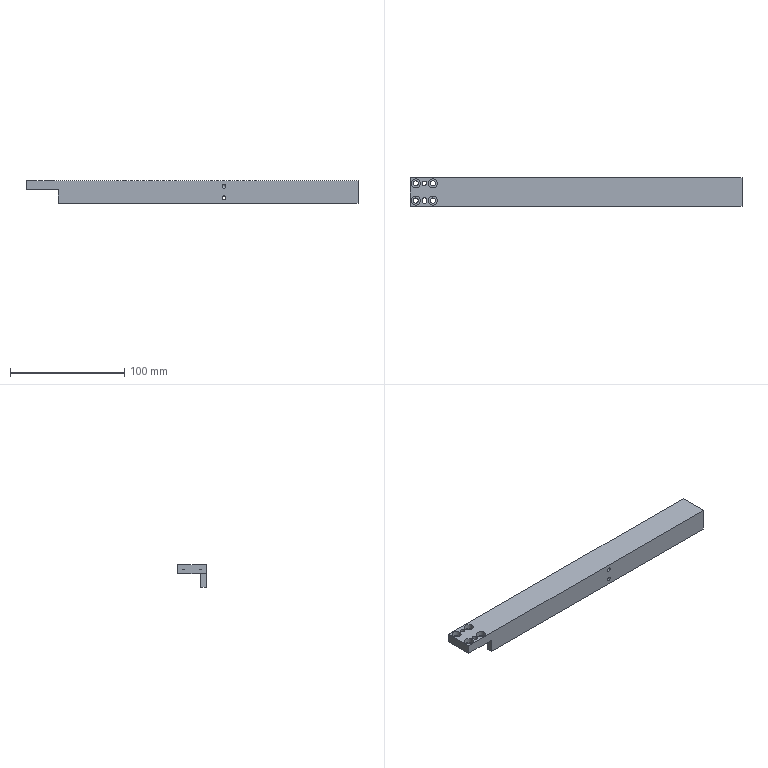Part | NX | 1 solid | 31 faces | box 290 x 25 x 20 mm | volume 71804 mm3 | plane 17 | cylinder 13 | cone 1 | commonest cylinder face diameters 4.5 x4 8 x4 4 x3 3.3 x2
STEP:
#1=CARTESIAN_POINT('',(-117.,-7.5,-20.));
#2=VERTEX_POINT('',#1);
#3=CARTESIAN_POINT('',(136.758,-7.5,-20.));
#4=VERTEX_POINT('',#3);
#5=CARTESIAN_POINT('',(-145.,-7.5,-20.));
#6=DIRECTION('',(1.,0.,0.));
#7=VECTOR('',#6,1000.);
#8=LINE('',#5,#7);
#9=EDGE_CURVE('',#2,#4,#8,.T.);
#10=ORIENTED_EDGE('',*,*,#9,.T.);
#11=CARTESIAN_POINT('',(145.,-10.5,-20.));
#12=VERTEX_POINT('',#11);
#13=CARTESIAN_POINT('',(136.758,-7.5,-20.));
#14=DIRECTION('',(0.9397,-0.342,0.));
#15=VECTOR('',#14,1000.);
#16=LINE('',#13,#15);
#17=EDGE_CURVE('',#4,#12,#16,.T.);
#18=ORIENTED_EDGE('',*,*,#17,.T.);
#19=CARTESIAN_POINT('',(145.,-12.5,-20.));
#20=VERTEX_POINT('',#19);
#21=CARTESIAN_POINT('',(145.,12.5,-20.));
#22=DIRECTION('',(0.,-1.,0.));
#23=VECTOR('',#22,1000.);
#24=LINE('',#21,#23);
#25=EDGE_CURVE('',#12,#20,#24,.T.);
#26=ORIENTED_EDGE('',*,*,#25,.T.);
#27=CARTESIAN_POINT('',(-117.,-12.5,-20.));
#28=VERTEX_POINT('',#27);
#29=CARTESIAN_POINT('',(145.,-12.5,-20.));
#30=DIRECTION('',(-1.,0.,0.));
#31=VECTOR('',#30,1000.);
#32=LINE('',#29,#31);
#33=EDGE_CURVE('',#20,#28,#32,.T.);
#34=ORIENTED_EDGE('',*,*,#33,.T.);
#35=CARTESIAN_POINT('',(-117.,-12.5,-20.));
#36=DIRECTION('',(0.,1.,0.));
#37=VECTOR('',#36,1000.);
#38=LINE('',#35,#37);
#39=EDGE_CURVE('',#28,#2,#38,.T.);
#40=ORIENTED_EDGE('',*,*,#39,.T.);
#41=EDGE_LOOP('',(#10,#18,#26,#34,#40));
#42=FACE_BOUND('',#41,.T.);
#43=CARTESIAN_POINT('',(145.,12.5,-20.));
#44=DIRECTION('',(0.,0.,1.));
#45=DIRECTION('',(-1.,0.,0.));
#46=AXIS2_PLACEMENT_3D('',#43,#44,#45);
#47=PLANE('',#46);
#48=ADVANCED_FACE('',(#42),#47,.F.);
#49=CARTESIAN_POINT('',(-145.,12.5,-8.));
#50=VERTEX_POINT('',#49);
#51=CARTESIAN_POINT('',(-145.,-12.5,-8.));
#52=VERTEX_POINT('',#51);
#53=CARTESIAN_POINT('',(-145.,-7.5,-8.));
#54=DIRECTION('',(0.,-1.,0.));
#55=VECTOR('',#54,1000.);
#56=LINE('',#53,#55);
#57=EDGE_CURVE('',#50,#52,#56,.T.);
#58=ORIENTED_EDGE('',*,*,#57,.T.);
#59=CARTESIAN_POINT('',(-145.,-12.5,0.));
#60=VERTEX_POINT('',#59);
#61=CARTESIAN_POINT('',(-145.,-12.5,-20.));
#62=DIRECTION('',(0.,0.,1.));
#63=VECTOR('',#62,1000.);
#64=LINE('',#61,#63);
#65=EDGE_CURVE('',#52,#60,#64,.T.);
#66=ORIENTED_EDGE('',*,*,#65,.T.);
#67=CARTESIAN_POINT('',(-145.,12.5,0.));
#68=VERTEX_POINT('',#67);
#69=CARTESIAN_POINT('',(-145.,12.5,0.));
#70=DIRECTION('',(0.,-1.,0.));
#71=VECTOR('',#70,1000.);
#72=LINE('',#69,#71);
#73=EDGE_CURVE('',#68,#60,#72,.T.);
#74=ORIENTED_EDGE('',*,*,#73,.F.);
#75=CARTESIAN_POINT('',(-145.,12.5,-20.));
#76=DIRECTION('',(0.,0.,1.));
#77=VECTOR('',#76,1000.);
#78=LINE('',#75,#77);
#79=EDGE_CURVE('',#50,#68,#78,.T.);
#80=ORIENTED_EDGE('',*,*,#79,.F.);
#81=EDGE_LOOP('',(#58,#66,#74,#80));
#82=FACE_BOUND('',#81,.T.);
#83=CARTESIAN_POINT('',(-145.,12.5,-20.));
#84=DIRECTION('',(1.,0.,0.));
#85=DIRECTION('',(0.,0.,1.));
#86=AXIS2_PLACEMENT_3D('',#83,#84,#85);
#87=PLANE('',#86);
#88=ADVANCED_FACE('',(#82),#87,.F.);
#89=CARTESIAN_POINT('',(-134.5,-7.,0.));
#90=VERTEX_POINT('',#89);
#91=CARTESIAN_POINT('',(-134.5,-8.,0.));
#92=VERTEX_POINT('',#91);
#93=CARTESIAN_POINT('',(-134.5,-7.,0.));
#94=DIRECTION('',(0.,-1.,0.));
#95=VECTOR('',#94,1000.);
#96=LINE('',#93,#95);
#97=EDGE_CURVE('',#90,#92,#96,.T.);
#98=ORIENTED_EDGE('',*,*,#97,.F.);
#99=CARTESIAN_POINT('',(-130.5,-7.,0.));
#100=VERTEX_POINT('',#99);
#101=CARTESIAN_POINT('',(-132.5,-7.,0.));
#102=DIRECTION('',(0.,0.,1.));
#103=DIRECTION('',(1.,0.,0.));
#104=AXIS2_PLACEMENT_3D('',#101,#102,#103);
#105=CIRCLE('',#104,2.);
#106=EDGE_CURVE('',#100,#90,#105,.T.);
#107=ORIENTED_EDGE('',*,*,#106,.F.);
#108=CARTESIAN_POINT('',(-130.5,-8.,0.));
#109=VERTEX_POINT('',#108);
#110=CARTESIAN_POINT('',(-130.5,-7.,0.));
#111=DIRECTION('',(0.,1.,0.));
#112=VECTOR('',#111,1000.);
#113=LINE('',#110,#112);
#114=EDGE_CURVE('',#109,#100,#113,.T.);
#115=ORIENTED_EDGE('',*,*,#114,.F.);
#116=CARTESIAN_POINT('',(-132.5,-8.,0.));
#117=DIRECTION('',(0.,0.,1.));
#118=DIRECTION('',(1.,0.,0.));
#119=AXIS2_PLACEMENT_3D('',#116,#117,#118);
#120=CIRCLE('',#119,2.);
#121=EDGE_CURVE('',#92,#109,#120,.T.);
#122=ORIENTED_EDGE('',*,*,#121,.F.);
#123=EDGE_LOOP('',(#98,#107,#115,#122));
#124=FACE_BOUND('',#123,.T.);
#125=CARTESIAN_POINT('',(-130.5,7.5,0.));
#126=VERTEX_POINT('',#125);
#127=CARTESIAN_POINT('',(-132.5,7.5,0.));
#128=DIRECTION('',(0.,0.,1.));
#129=DIRECTION('',(1.,0.,0.));
#130=AXIS2_PLACEMENT_3D('',#127,#128,#129);
#131=CIRCLE('',#130,2.);
#132=EDGE_CURVE('',#126,#126,#131,.T.);
#133=ORIENTED_EDGE('',*,*,#132,.F.);
#134=EDGE_LOOP('',(#133));
#135=FACE_BOUND('',#134,.T.);
#136=CARTESIAN_POINT('',(-136.,7.5,0.));
#137=VERTEX_POINT('',#136);
#138=CARTESIAN_POINT('',(-140.,7.5,0.));
#139=DIRECTION('',(0.,0.,1.));
#140=DIRECTION('',(1.,0.,0.));
#141=AXIS2_PLACEMENT_3D('',#138,#139,#140);
#142=CIRCLE('',#141,4.);
#143=EDGE_CURVE('',#137,#137,#142,.T.);
#144=ORIENTED_EDGE('',*,*,#143,.F.);
#145=EDGE_LOOP('',(#144));
#146=FACE_BOUND('',#145,.T.);
#147=CARTESIAN_POINT('',(-136.,-7.5,0.));
#148=VERTEX_POINT('',#147);
#149=CARTESIAN_POINT('',(-140.,-7.5,0.));
#150=DIRECTION('',(0.,0.,1.));
#151=DIRECTION('',(1.,0.,0.));
#152=AXIS2_PLACEMENT_3D('',#149,#150,#151);
#153=CIRCLE('',#152,4.);
#154=EDGE_CURVE('',#148,#148,#153,.T.);
#155=ORIENTED_EDGE('',*,*,#154,.F.);
#156=EDGE_LOOP('',(#155));
#157=FACE_BOUND('',#156,.T.);
#158=CARTESIAN_POINT('',(-121.,-7.5,0.));
#159=VERTEX_POINT('',#158);
#160=CARTESIAN_POINT('',(-125.,-7.5,0.));
#161=DIRECTION('',(0.,0.,1.));
#162=DIRECTION('',(1.,0.,0.));
#163=AXIS2_PLACEMENT_3D('',#160,#161,#162);
#164=CIRCLE('',#163,4.);
#165=EDGE_CURVE('',#159,#159,#164,.T.);
#166=ORIENTED_EDGE('',*,*,#165,.F.);
#167=EDGE_LOOP('',(#166));
#168=FACE_BOUND('',#167,.T.);
#169=CARTESIAN_POINT('',(-121.,7.5,0.));
#170=VERTEX_POINT('',#169);
#171=CARTESIAN_POINT('',(-125.,7.5,0.));
#172=DIRECTION('',(0.,0.,1.));
#173=DIRECTION('',(1.,0.,0.));
#174=AXIS2_PLACEMENT_3D('',#171,#172,#173);
#175=CIRCLE('',#174,4.);
#176=EDGE_CURVE('',#170,#170,#175,.T.);
#177=ORIENTED_EDGE('',*,*,#176,.F.);
#178=EDGE_LOOP('',(#177));
#179=FACE_BOUND('',#178,.T.);
#180=CARTESIAN_POINT('',(145.,-12.5,0.));
#181=VERTEX_POINT('',#180);
#182=CARTESIAN_POINT('',(145.,-12.5,0.));
#183=DIRECTION('',(1.,0.,0.));
#184=VECTOR('',#183,1000.);
#185=LINE('',#182,#184);
#186=EDGE_CURVE('',#60,#181,#185,.T.);
#187=ORIENTED_EDGE('',*,*,#186,.T.);
#188=CARTESIAN_POINT('',(145.,12.5,0.));
#189=VERTEX_POINT('',#188);
#190=CARTESIAN_POINT('',(145.,12.5,0.));
#191=DIRECTION('',(0.,-1.,0.));
#192=VECTOR('',#191,1000.);
#193=LINE('',#190,#192);
#194=EDGE_CURVE('',#189,#181,#193,.T.);
#195=ORIENTED_EDGE('',*,*,#194,.F.);
#196=CARTESIAN_POINT('',(145.,12.5,0.));
#197=DIRECTION('',(1.,0.,0.));
#198=VECTOR('',#197,1000.);
#199=LINE('',#196,#198);
#200=EDGE_CURVE('',#68,#189,#199,.T.);
#201=ORIENTED_EDGE('',*,*,#200,.F.);
#202=ORIENTED_EDGE('',*,*,#73,.T.);
#203=EDGE_LOOP('',(#187,#195,#201,#202));
#204=FACE_BOUND('',#203,.T.);
#205=CARTESIAN_POINT('',(145.,12.5,0.));
#206=DIRECTION('',(0.,0.,-1.));
#207=DIRECTION('',(1.,0.,0.));
#208=AXIS2_PLACEMENT_3D('',#205,#206,#207);
#209=PLANE('',#208);
#210=ADVANCED_FACE('',(#124,#135,#146,#157,#168,#179,#204),#209,.F.);
#211=ORIENTED_EDGE('',*,*,#25,.F.);
#212=CARTESIAN_POINT('',(145.,-10.5,-5.));
#213=VERTEX_POINT('',#212);
#214=CARTESIAN_POINT('',(145.,-10.5,-20.));
#215=DIRECTION('',(0.,0.,1.));
#216=VECTOR('',#215,1000.);
#217=LINE('',#214,#216);
#218=EDGE_CURVE('',#12,#213,#217,.T.);
#219=ORIENTED_EDGE('',*,*,#218,.T.);
#220=CARTESIAN_POINT('',(145.,12.5,-5.));
#221=VERTEX_POINT('',#220);
#222=CARTESIAN_POINT('',(145.,12.5,-5.));
#223=DIRECTION('',(0.,1.,0.));
#224=VECTOR('',#223,1000.);
#225=LINE('',#222,#224);
#226=EDGE_CURVE('',#213,#221,#225,.T.);
#227=ORIENTED_EDGE('',*,*,#226,.T.);
#228=CARTESIAN_POINT('',(145.,12.5,-20.));
#229=DIRECTION('',(0.,0.,-1.));
#230=VECTOR('',#229,1000.);
#231=LINE('',#228,#230);
#232=EDGE_CURVE('',#189,#221,#231,.T.);
#233=ORIENTED_EDGE('',*,*,#232,.F.);
#234=ORIENTED_EDGE('',*,*,#194,.T.);
#235=CARTESIAN_POINT('',(145.,-12.5,-20.));
#236=DIRECTION('',(0.,0.,-1.));
#237=VECTOR('',#236,1000.);
#238=LINE('',#235,#237);
#239=EDGE_CURVE('',#181,#20,#238,.T.);
#240=ORIENTED_EDGE('',*,*,#239,.T.);
#241=EDGE_LOOP('',(#211,#219,#227,#233,#234,#240));
#242=FACE_BOUND('',#241,.T.);
#243=CARTESIAN_POINT('',(145.,12.5,-20.));
#244=DIRECTION('',(-1.,0.,0.));
#245=DIRECTION('',(0.,0.,-1.));
#246=AXIS2_PLACEMENT_3D('',#243,#244,#245);
#247=PLANE('',#246);
#248=ADVANCED_FACE('',(#242),#247,.F.);
#249=ORIENTED_EDGE('',*,*,#232,.T.);
#250=CARTESIAN_POINT('',(136.758,12.5,-8.));
#251=VERTEX_POINT('',#250);
#252=CARTESIAN_POINT('',(-115.897,12.5,-99.959));
#253=DIRECTION('',(-0.9397,0.,-0.342));
#254=VECTOR('',#253,1000.);
#255=LINE('',#252,#254);
#256=EDGE_CURVE('',#221,#251,#255,.T.);
#257=ORIENTED_EDGE('',*,*,#256,.T.);
#258=CARTESIAN_POINT('',(-145.,12.5,-8.));
#259=DIRECTION('',(1.,0.,0.));
#260=VECTOR('',#259,1000.);
#261=LINE('',#258,#260);
#262=EDGE_CURVE('',#50,#251,#261,.T.);
#263=ORIENTED_EDGE('',*,*,#262,.F.);
#264=ORIENTED_EDGE('',*,*,#79,.T.);
#265=ORIENTED_EDGE('',*,*,#200,.T.);
#266=EDGE_LOOP('',(#249,#257,#263,#264,#265));
#267=FACE_BOUND('',#266,.T.);
#268=CARTESIAN_POINT('',(-145.,12.5,-20.));
#269=DIRECTION('',(0.,1.,0.));
#270=DIRECTION('',(1.,0.,0.));
#271=AXIS2_PLACEMENT_3D('',#268,#269,#270);
#272=PLANE('',#271);
#273=ADVANCED_FACE('',(#267),#272,.T.);
#274=CARTESIAN_POINT('',(29.65,-12.5,-5.));
#275=VERTEX_POINT('',#274);
#276=CARTESIAN_POINT('',(28.,-12.5,-5.));
#277=DIRECTION('',(0.,-1.,0.));
#278=DIRECTION('',(1.,0.,0.));
#279=AXIS2_PLACEMENT_3D('',#276,#277,#278);
#280=CIRCLE('',#279,1.65);
#281=EDGE_CURVE('',#275,#275,#280,.T.);
#282=ORIENTED_EDGE('',*,*,#281,.F.);
#283=EDGE_LOOP('',(#282));
#284=FACE_BOUND('',#283,.T.);
#285=CARTESIAN_POINT('',(29.65,-12.5,-15.));
#286=VERTEX_POINT('',#285);
#287=CARTESIAN_POINT('',(28.,-12.5,-15.));
#288=DIRECTION('',(0.,-1.,0.));
#289=DIRECTION('',(1.,0.,0.));
#290=AXIS2_PLACEMENT_3D('',#287,#288,#289);
#291=CIRCLE('',#290,1.65);
#292=EDGE_CURVE('',#286,#286,#291,.T.);
#293=ORIENTED_EDGE('',*,*,#292,.F.);
#294=EDGE_LOOP('',(#293));
#295=FACE_BOUND('',#294,.T.);
#296=CARTESIAN_POINT('',(-117.,-12.5,-8.));
#297=VERTEX_POINT('',#296);
#298=CARTESIAN_POINT('',(-145.,-12.5,-8.));
#299=DIRECTION('',(1.,0.,0.));
#300=VECTOR('',#299,1000.);
#301=LINE('',#298,#300);
#302=EDGE_CURVE('',#52,#297,#301,.T.);
#303=ORIENTED_EDGE('',*,*,#302,.T.);
#304=CARTESIAN_POINT('',(-117.,-12.5,-20.));
#305=DIRECTION('',(0.,0.,-1.));
#306=VECTOR('',#305,1000.);
#307=LINE('',#304,#306);
#308=EDGE_CURVE('',#297,#28,#307,.T.);
#309=ORIENTED_EDGE('',*,*,#308,.T.);
#310=ORIENTED_EDGE('',*,*,#33,.F.);
#311=ORIENTED_EDGE('',*,*,#239,.F.);
#312=ORIENTED_EDGE('',*,*,#186,.F.);
#313=ORIENTED_EDGE('',*,*,#65,.F.);
#314=EDGE_LOOP('',(#303,#309,#310,#311,#312,#313));
#315=FACE_BOUND('',#314,.T.);
#316=CARTESIAN_POINT('',(-145.,-12.5,-20.));
#317=DIRECTION('',(0.,1.,0.));
#318=DIRECTION('',(1.,0.,0.));
#319=AXIS2_PLACEMENT_3D('',#316,#317,#318);
#320=PLANE('',#319);
#321=ADVANCED_FACE('',(#284,#295,#315),#320,.F.);
#322=CARTESIAN_POINT('',(28.,-7.5,-13.35));
#323=VERTEX_POINT('',#322);
#324=CARTESIAN_POINT('',(28.,-7.5,-15.));
#325=DIRECTION('',(0.,-1.,0.));
#326=DIRECTION('',(0.,0.,1.));
#327=AXIS2_PLACEMENT_3D('',#324,#325,#326);
#328=CIRCLE('',#327,1.65);
#329=EDGE_CURVE('',#323,#323,#328,.T.);
#330=ORIENTED_EDGE('',*,*,#329,.T.);
#331=EDGE_LOOP('',(#330));
#332=FACE_BOUND('',#331,.T.);
#333=CARTESIAN_POINT('',(-117.,-7.5,-8.));
#334=VERTEX_POINT('',#333);
#335=CARTESIAN_POINT('',(136.758,-7.5,-8.));
#336=VERTEX_POINT('',#335);
#337=CARTESIAN_POINT('',(-145.,-7.5,-8.));
#338=DIRECTION('',(1.,0.,0.));
#339=VECTOR('',#338,1000.);
#340=LINE('',#337,#339);
#341=EDGE_CURVE('',#334,#336,#340,.T.);
#342=ORIENTED_EDGE('',*,*,#341,.T.);
#343=CARTESIAN_POINT('',(136.758,-7.5,-20.));
#344=DIRECTION('',(0.,0.,-1.));
#345=VECTOR('',#344,1000.);
#346=LINE('',#343,#345);
#347=EDGE_CURVE('',#336,#4,#346,.T.);
#348=ORIENTED_EDGE('',*,*,#347,.T.);
#349=ORIENTED_EDGE('',*,*,#9,.F.);
#350=CARTESIAN_POINT('',(-117.,-7.5,-20.));
#351=DIRECTION('',(0.,0.,1.));
#352=VECTOR('',#351,1000.);
#353=LINE('',#350,#352);
#354=EDGE_CURVE('',#2,#334,#353,.T.);
#355=ORIENTED_EDGE('',*,*,#354,.T.);
#356=EDGE_LOOP('',(#342,#348,#349,#355));
#357=FACE_BOUND('',#356,.T.);
#358=CARTESIAN_POINT('',(-145.,-7.5,-20.));
#359=DIRECTION('',(0.,-1.,0.));
#360=DIRECTION('',(0.,0.,-1.));
#361=AXIS2_PLACEMENT_3D('',#358,#359,#360);
#362=PLANE('',#361);
#363=ADVANCED_FACE('',(#332,#357),#362,.F.);
#364=CARTESIAN_POINT('',(-130.5,-8.,-8.));
#365=VERTEX_POINT('',#364);
#366=CARTESIAN_POINT('',(-130.5,-7.,-8.));
#367=VERTEX_POINT('',#366);
#368=CARTESIAN_POINT('',(-130.5,-7.5,-8.));
#369=DIRECTION('',(0.,1.,0.));
#370=VECTOR('',#369,1000.);
#371=LINE('',#368,#370);
#372=EDGE_CURVE('',#365,#367,#371,.T.);
#373=ORIENTED_EDGE('',*,*,#372,.T.);
#374=CARTESIAN_POINT('',(-134.5,-7.,-8.));
#375=VERTEX_POINT('',#374);
#376=CARTESIAN_POINT('',(-132.5,-7.,-8.));
#377=DIRECTION('',(0.,0.,1.));
#378=DIRECTION('',(0.,1.,0.));
#379=AXIS2_PLACEMENT_3D('',#376,#377,#378);
#380=CIRCLE('',#379,2.);
#381=EDGE_CURVE('',#367,#375,#380,.T.);
#382=ORIENTED_EDGE('',*,*,#381,.T.);
#383=CARTESIAN_POINT('',(-134.5,-8.,-8.));
#384=VERTEX_POINT('',#383);
#385=CARTESIAN_POINT('',(-134.5,-7.5,-8.));
#386=DIRECTION('',(0.,-1.,0.));
#387=VECTOR('',#386,1000.);
#388=LINE('',#385,#387);
#389=EDGE_CURVE('',#375,#384,#388,.T.);
#390=ORIENTED_EDGE('',*,*,#389,.T.);
#391=CARTESIAN_POINT('',(-132.5,-8.,-8.));
#392=DIRECTION('',(0.,0.,1.));
#393=DIRECTION('',(0.,1.,0.));
#394=AXIS2_PLACEMENT_3D('',#391,#392,#393);
#395=CIRCLE('',#394,2.);
#396=EDGE_CURVE('',#384,#365,#395,.T.);
#397=ORIENTED_EDGE('',*,*,#396,.T.);
#398=EDGE_LOOP('',(#373,#382,#390,#397));
#399=FACE_BOUND('',#398,.T.);
#400=CARTESIAN_POINT('',(-132.5,9.5,-8.));
#401=VERTEX_POINT('',#400);
#402=CARTESIAN_POINT('',(-132.5,7.5,-8.));
#403=DIRECTION('',(0.,0.,1.));
#404=DIRECTION('',(0.,1.,0.));
#405=AXIS2_PLACEMENT_3D('',#402,#403,#404);
#406=CIRCLE('',#405,2.);
#407=EDGE_CURVE('',#401,#401,#406,.T.);
#408=ORIENTED_EDGE('',*,*,#407,.T.);
#409=EDGE_LOOP('',(#408));
#410=FACE_BOUND('',#409,.T.);
#411=CARTESIAN_POINT('',(-140.,9.75,-8.));
#412=VERTEX_POINT('',#411);
#413=CARTESIAN_POINT('',(-140.,7.5,-8.));
#414=DIRECTION('',(0.,0.,1.));
#415=DIRECTION('',(0.,1.,0.));
#416=AXIS2_PLACEMENT_3D('',#413,#414,#415);
#417=CIRCLE('',#416,2.25);
#418=EDGE_CURVE('',#412,#412,#417,.T.);
#419=ORIENTED_EDGE('',*,*,#418,.T.);
#420=EDGE_LOOP('',(#419));
#421=FACE_BOUND('',#420,.T.);
#422=CARTESIAN_POINT('',(-140.,-5.25,-8.));
#423=VERTEX_POINT('',#422);
#424=CARTESIAN_POINT('',(-140.,-7.5,-8.));
#425=DIRECTION('',(0.,0.,1.));
#426=DIRECTION('',(0.,1.,0.));
#427=AXIS2_PLACEMENT_3D('',#424,#425,#426);
#428=CIRCLE('',#427,2.25);
#429=EDGE_CURVE('',#423,#423,#428,.T.);
#430=ORIENTED_EDGE('',*,*,#429,.T.);
#431=EDGE_LOOP('',(#430));
#432=FACE_BOUND('',#431,.T.);
#433=CARTESIAN_POINT('',(-125.,-5.25,-8.));
#434=VERTEX_POINT('',#433);
#435=CARTESIAN_POINT('',(-125.,-7.5,-8.));
#436=DIRECTION('',(0.,0.,1.));
#437=DIRECTION('',(0.,1.,0.));
#438=AXIS2_PLACEMENT_3D('',#435,#436,#437);
#439=CIRCLE('',#438,2.25);
#440=EDGE_CURVE('',#434,#434,#439,.T.);
#441=ORIENTED_EDGE('',*,*,#440,.T.);
#442=EDGE_LOOP('',(#441));
#443=FACE_BOUND('',#442,.T.);
#444=CARTESIAN_POINT('',(-125.,9.75,-8.));
#445=VERTEX_POINT('',#444);
#446=CARTESIAN_POINT('',(-125.,7.5,-8.));
#447=DIRECTION('',(0.,0.,1.));
#448=DIRECTION('',(0.,1.,0.));
#449=AXIS2_PLACEMENT_3D('',#446,#447,#448);
#450=CIRCLE('',#449,2.25);
#451=EDGE_CURVE('',#445,#445,#450,.T.);
#452=ORIENTED_EDGE('',*,*,#451,.T.);
#453=EDGE_LOOP('',(#452));
#454=FACE_BOUND('',#453,.T.);
#455=ORIENTED_EDGE('',*,*,#262,.T.);
#456=CARTESIAN_POINT('',(136.758,-7.5,-8.));
#457=DIRECTION('',(0.,-1.,0.));
#458=VECTOR('',#457,1000.);
#459=LINE('',#456,#458);
#460=EDGE_CURVE('',#251,#336,#459,.T.);
#461=ORIENTED_EDGE('',*,*,#460,.T.);
#462=ORIENTED_EDGE('',*,*,#341,.F.);
#463=CARTESIAN_POINT('',(-117.,-12.5,-8.));
#464=DIRECTION('',(0.,1.,0.));
#465=VECTOR('',#464,1000.);
#466=LINE('',#463,#465);
#467=EDGE_CURVE('',#297,#334,#466,.T.);
#468=ORIENTED_EDGE('',*,*,#467,.F.);
#469=ORIENTED_EDGE('',*,*,#302,.F.);
#470=ORIENTED_EDGE('',*,*,#57,.F.);
#471=EDGE_LOOP('',(#455,#461,#462,#468,#469,#470));
#472=FACE_BOUND('',#471,.T.);
#473=CARTESIAN_POINT('',(-145.,-7.5,-8.));
#474=DIRECTION('',(0.,0.,1.));
#475=DIRECTION('',(0.,-1.,0.));
#476=AXIS2_PLACEMENT_3D('',#473,#474,#475);
#477=PLANE('',#476);
#478=ADVANCED_FACE('',(#399,#410,#421,#432,#443,#454,#472),#477,.F.);
#479=ORIENTED_EDGE('',*,*,#39,.F.);
#480=ORIENTED_EDGE('',*,*,#308,.F.);
#481=ORIENTED_EDGE('',*,*,#467,.T.);
#482=ORIENTED_EDGE('',*,*,#354,.F.);
#483=EDGE_LOOP('',(#479,#480,#481,#482));
#484=FACE_BOUND('',#483,.T.);
#485=CARTESIAN_POINT('',(-117.,-12.5,-20.));
#486=DIRECTION('',(1.,0.,0.));
#487=DIRECTION('',(0.,0.,1.));
#488=AXIS2_PLACEMENT_3D('',#485,#486,#487);
#489=PLANE('',#488);
#490=ADVANCED_FACE('',(#484),#489,.F.);
#491=CARTESIAN_POINT('',(-122.75,7.5,-4.4));
#492=VERTEX_POINT('',#491);
#493=CARTESIAN_POINT('',(-125.,7.5,-4.4));
#494=DIRECTION('',(0.,0.,1.));
#495=DIRECTION('',(1.,0.,0.));
#496=AXIS2_PLACEMENT_3D('',#493,#494,#495);
#497=CIRCLE('',#496,2.25);
#498=EDGE_CURVE('',#492,#492,#497,.T.);
#499=ORIENTED_EDGE('',*,*,#498,.T.);
#500=EDGE_LOOP('',(#499));
#501=FACE_BOUND('',#500,.T.);
#502=ORIENTED_EDGE('',*,*,#451,.F.);
#503=EDGE_LOOP('',(#502));
#504=FACE_BOUND('',#503,.T.);
#505=CARTESIAN_POINT('',(-125.,7.5,0.));
#506=DIRECTION('',(0.,0.,1.));
#507=DIRECTION('',(-1.,0.,0.));
#508=AXIS2_PLACEMENT_3D('',#505,#506,#507);
#509=CYLINDRICAL_SURFACE('',#508,2.25);
#510=ADVANCED_FACE('',(#501,#504),#509,.F.);
#511=ORIENTED_EDGE('',*,*,#498,.F.);
#512=EDGE_LOOP('',(#511));
#513=FACE_BOUND('',#512,.T.);
#514=CARTESIAN_POINT('',(-121.,7.5,-4.4));
#515=VERTEX_POINT('',#514);
#516=CARTESIAN_POINT('',(-125.,7.5,-4.4));
#517=DIRECTION('',(0.,0.,1.));
#518=DIRECTION('',(1.,0.,0.));
#519=AXIS2_PLACEMENT_3D('',#516,#517,#518);
#520=CIRCLE('',#519,4.);
#521=EDGE_CURVE('',#515,#515,#520,.T.);
#522=ORIENTED_EDGE('',*,*,#521,.T.);
#523=EDGE_LOOP('',(#522));
#524=FACE_BOUND('',#523,.T.);
#525=CARTESIAN_POINT('',(-125.,9.75,-4.4));
#526=DIRECTION('',(0.,0.,-1.));
#527=DIRECTION('',(1.,0.,0.));
#528=AXIS2_PLACEMENT_3D('',#525,#526,#527);
#529=PLANE('',#528);
#530=ADVANCED_FACE('',(#513,#524),#529,.F.);
#531=ORIENTED_EDGE('',*,*,#521,.F.);
#532=EDGE_LOOP('',(#531));
#533=FACE_BOUND('',#532,.T.);
#534=ORIENTED_EDGE('',*,*,#176,.T.);
#535=EDGE_LOOP('',(#534));
#536=FACE_BOUND('',#535,.T.);
#537=CARTESIAN_POINT('',(-125.,7.5,0.));
#538=DIRECTION('',(0.,0.,1.));
#539=DIRECTION('',(-1.,0.,0.));
#540=AXIS2_PLACEMENT_3D('',#537,#538,#539);
#541=CYLINDRICAL_SURFACE('',#540,4.);
#542=ADVANCED_FACE('',(#533,#536),#541,.F.);
#543=CARTESIAN_POINT('',(-122.75,-7.5,-4.4));
#544=VERTEX_POINT('',#543);
#545=CARTESIAN_POINT('',(-125.,-7.5,-4.4));
#546=DIRECTION('',(0.,0.,1.));
#547=DIRECTION('',(1.,0.,0.));
#548=AXIS2_PLACEMENT_3D('',#545,#546,#547);
#549=CIRCLE('',#548,2.25);
#550=EDGE_CURVE('',#544,#544,#549,.T.);
#551=ORIENTED_EDGE('',*,*,#550,.T.);
#552=EDGE_LOOP('',(#551));
#553=FACE_BOUND('',#552,.T.);
#554=ORIENTED_EDGE('',*,*,#440,.F.);
#555=EDGE_LOOP('',(#554));
#556=FACE_BOUND('',#555,.T.);
#557=CARTESIAN_POINT('',(-125.,-7.5,0.));
#558=DIRECTION('',(0.,0.,1.));
#559=DIRECTION('',(-1.,0.,0.));
#560=AXIS2_PLACEMENT_3D('',#557,#558,#559);
#561=CYLINDRICAL_SURFACE('',#560,2.25);
#562=ADVANCED_FACE('',(#553,#556),#561,.F.);
#563=ORIENTED_EDGE('',*,*,#550,.F.);
#564=EDGE_LOOP('',(#563));
#565=FACE_BOUND('',#564,.T.);
#566=CARTESIAN_POINT('',(-121.,-7.5,-4.4));
#567=VERTEX_POINT('',#566);
#568=CARTESIAN_POINT('',(-125.,-7.5,-4.4));
#569=DIRECTION('',(0.,0.,1.));
#570=DIRECTION('',(1.,0.,0.));
#571=AXIS2_PLACEMENT_3D('',#568,#569,#570);
#572=CIRCLE('',#571,4.);
#573=EDGE_CURVE('',#567,#567,#572,.T.);
#574=ORIENTED_EDGE('',*,*,#573,.T.);
#575=EDGE_LOOP('',(#574));
#576=FACE_BOUND('',#575,.T.);
#577=CARTESIAN_POINT('',(-125.,-5.25,-4.4));
#578=DIRECTION('',(0.,0.,-1.));
#579=DIRECTION('',(1.,0.,0.));
#580=AXIS2_PLACEMENT_3D('',#577,#578,#579);
#581=PLANE('',#580);
#582=ADVANCED_FACE('',(#565,#576),#581,.F.);
#583=ORIENTED_EDGE('',*,*,#573,.F.);
#584=EDGE_LOOP('',(#583));
#585=FACE_BOUND('',#584,.T.);
#586=ORIENTED_EDGE('',*,*,#165,.T.);
#587=EDGE_LOOP('',(#586));
#588=FACE_BOUND('',#587,.T.);
#589=CARTESIAN_POINT('',(-125.,-7.5,0.));
#590=DIRECTION('',(0.,0.,1.));
#591=DIRECTION('',(-1.,0.,0.));
#592=AXIS2_PLACEMENT_3D('',#589,#590,#591);
#593=CYLINDRICAL_SURFACE('',#592,4.);
#594=ADVANCED_FACE('',(#585,#588),#593,.F.);
#595=CARTESIAN_POINT('',(-137.75,-7.5,-4.4));
#596=VERTEX_POINT('',#595);
#597=CARTESIAN_POINT('',(-140.,-7.5,-4.4));
#598=DIRECTION('',(0.,0.,1.));
#599=DIRECTION('',(1.,0.,0.));
#600=AXIS2_PLACEMENT_3D('',#597,#598,#599);
#601=CIRCLE('',#600,2.25);
#602=EDGE_CURVE('',#596,#596,#601,.T.);
#603=ORIENTED_EDGE('',*,*,#602,.T.);
#604=EDGE_LOOP('',(#603));
#605=FACE_BOUND('',#604,.T.);
#606=ORIENTED_EDGE('',*,*,#429,.F.);
#607=EDGE_LOOP('',(#606));
#608=FACE_BOUND('',#607,.T.);
#609=CARTESIAN_POINT('',(-140.,-7.5,0.));
#610=DIRECTION('',(0.,0.,1.));
#611=DIRECTION('',(-1.,0.,0.));
#612=AXIS2_PLACEMENT_3D('',#609,#610,#611);
#613=CYLINDRICAL_SURFACE('',#612,2.25);
#614=ADVANCED_FACE('',(#605,#608),#613,.F.);
#615=ORIENTED_EDGE('',*,*,#602,.F.);
#616=EDGE_LOOP('',(#615));
#617=FACE_BOUND('',#616,.T.);
#618=CARTESIAN_POINT('',(-136.,-7.5,-4.4));
#619=VERTEX_POINT('',#618);
#620=CARTESIAN_POINT('',(-140.,-7.5,-4.4));
#621=DIRECTION('',(0.,0.,1.));
#622=DIRECTION('',(1.,0.,0.));
#623=AXIS2_PLACEMENT_3D('',#620,#621,#622);
#624=CIRCLE('',#623,4.);
#625=EDGE_CURVE('',#619,#619,#624,.T.);
#626=ORIENTED_EDGE('',*,*,#625,.T.);
#627=EDGE_LOOP('',(#626));
#628=FACE_BOUND('',#627,.T.);
#629=CARTESIAN_POINT('',(-140.,-5.25,-4.4));
#630=DIRECTION('',(0.,0.,-1.));
#631=DIRECTION('',(1.,0.,0.));
#632=AXIS2_PLACEMENT_3D('',#629,#630,#631);
#633=PLANE('',#632);
#634=ADVANCED_FACE('',(#617,#628),#633,.F.);
#635=ORIENTED_EDGE('',*,*,#625,.F.);
#636=EDGE_LOOP('',(#635));
#637=FACE_BOUND('',#636,.T.);
#638=ORIENTED_EDGE('',*,*,#154,.T.);
#639=EDGE_LOOP('',(#638));
#640=FACE_BOUND('',#639,.T.);
#641=CARTESIAN_POINT('',(-140.,-7.5,0.));
#642=DIRECTION('',(0.,0.,1.));
#643=DIRECTION('',(-1.,0.,0.));
#644=AXIS2_PLACEMENT_3D('',#641,#642,#643);
#645=CYLINDRICAL_SURFACE('',#644,4.);
#646=ADVANCED_FACE('',(#637,#640),#645,.F.);
#647=CARTESIAN_POINT('',(-137.75,7.5,-4.4));
#648=VERTEX_POINT('',#647);
#649=CARTESIAN_POINT('',(-140.,7.5,-4.4));
#650=DIRECTION('',(0.,0.,1.));
#651=DIRECTION('',(1.,0.,0.));
#652=AXIS2_PLACEMENT_3D('',#649,#650,#651);
#653=CIRCLE('',#652,2.25);
#654=EDGE_CURVE('',#648,#648,#653,.T.);
#655=ORIENTED_EDGE('',*,*,#654,.T.);
#656=EDGE_LOOP('',(#655));
#657=FACE_BOUND('',#656,.T.);
#658=ORIENTED_EDGE('',*,*,#418,.F.);
#659=EDGE_LOOP('',(#658));
#660=FACE_BOUND('',#659,.T.);
#661=CARTESIAN_POINT('',(-140.,7.5,0.));
#662=DIRECTION('',(0.,0.,1.));
#663=DIRECTION('',(-1.,0.,0.));
#664=AXIS2_PLACEMENT_3D('',#661,#662,#663);
#665=CYLINDRICAL_SURFACE('',#664,2.25);
#666=ADVANCED_FACE('',(#657,#660),#665,.F.);
#667=ORIENTED_EDGE('',*,*,#654,.F.);
#668=EDGE_LOOP('',(#667));
#669=FACE_BOUND('',#668,.T.);
#670=CARTESIAN_POINT('',(-136.,7.5,-4.4));
#671=VERTEX_POINT('',#670);
#672=CARTESIAN_POINT('',(-140.,7.5,-4.4));
#673=DIRECTION('',(0.,0.,1.));
#674=DIRECTION('',(1.,0.,0.));
#675=AXIS2_PLACEMENT_3D('',#672,#673,#674);
#676=CIRCLE('',#675,4.);
#677=EDGE_CURVE('',#671,#671,#676,.T.);
#678=ORIENTED_EDGE('',*,*,#677,.T.);
#679=EDGE_LOOP('',(#678));
#680=FACE_BOUND('',#679,.T.);
#681=CARTESIAN_POINT('',(-140.,9.75,-4.4));
#682=DIRECTION('',(0.,0.,-1.));
#683=DIRECTION('',(1.,0.,0.));
#684=AXIS2_PLACEMENT_3D('',#681,#682,#683);
#685=PLANE('',#684);
#686=ADVANCED_FACE('',(#669,#680),#685,.F.);
#687=ORIENTED_EDGE('',*,*,#677,.F.);
#688=EDGE_LOOP('',(#687));
#689=FACE_BOUND('',#688,.T.);
#690=ORIENTED_EDGE('',*,*,#143,.T.);
#691=EDGE_LOOP('',(#690));
#692=FACE_BOUND('',#691,.T.);
#693=CARTESIAN_POINT('',(-140.,7.5,0.));
#694=DIRECTION('',(0.,0.,1.));
#695=DIRECTION('',(-1.,0.,0.));
#696=AXIS2_PLACEMENT_3D('',#693,#694,#695);
#697=CYLINDRICAL_SURFACE('',#696,4.);
#698=ADVANCED_FACE('',(#689,#692),#697,.F.);
#699=ORIENTED_EDGE('',*,*,#256,.F.);
#700=ORIENTED_EDGE('',*,*,#226,.F.);
#701=CARTESIAN_POINT('',(133.305,-6.243,-9.257));
#702=DIRECTION('',(0.8891,-0.3236,0.3236));
#703=VECTOR('',#702,1000.);
#704=LINE('',#701,#703);
#705=EDGE_CURVE('',#336,#213,#704,.T.);
#706=ORIENTED_EDGE('',*,*,#705,.F.);
#707=ORIENTED_EDGE('',*,*,#460,.F.);
#708=EDGE_LOOP('',(#699,#700,#706,#707));
#709=FACE_BOUND('',#708,.T.);
#710=CARTESIAN_POINT('',(136.758,-7.5,-8.));
#711=DIRECTION('',(-0.342,0.,0.9397));
#712=DIRECTION('',(0.,1.,0.));
#713=AXIS2_PLACEMENT_3D('',#710,#711,#712);
#714=PLANE('',#713);
#715=ADVANCED_FACE('',(#709),#714,.F.);
#716=ORIENTED_EDGE('',*,*,#705,.T.);
#717=ORIENTED_EDGE('',*,*,#218,.F.);
#718=ORIENTED_EDGE('',*,*,#17,.F.);
#719=ORIENTED_EDGE('',*,*,#347,.F.);
#720=EDGE_LOOP('',(#716,#717,#718,#719));
#721=FACE_BOUND('',#720,.T.);
#722=CARTESIAN_POINT('',(136.758,-7.5,-20.));
#723=DIRECTION('',(-0.342,-0.9397,0.));
#724=DIRECTION('',(0.,0.,1.));
#725=AXIS2_PLACEMENT_3D('',#722,#723,#724);
#726=PLANE('',#725);
#727=ADVANCED_FACE('',(#721),#726,.F.);
#728=ORIENTED_EDGE('',*,*,#132,.T.);
#729=EDGE_LOOP('',(#728));
#730=FACE_BOUND('',#729,.T.);
#731=ORIENTED_EDGE('',*,*,#407,.F.);
#732=EDGE_LOOP('',(#731));
#733=FACE_BOUND('',#732,.T.);
#734=CARTESIAN_POINT('',(-132.5,7.5,-20.));
#735=DIRECTION('',(0.,0.,1.));
#736=DIRECTION('',(-1.,0.,0.));
#737=AXIS2_PLACEMENT_3D('',#734,#735,#736);
#738=CYLINDRICAL_SURFACE('',#737,2.);
#739=ADVANCED_FACE('',(#730,#733),#738,.F.);
#740=CARTESIAN_POINT('',(-130.5,-7.,-20.));
#741=DIRECTION('',(0.,0.,1.));
#742=VECTOR('',#741,1000.);
#743=LINE('',#740,#742);
#744=EDGE_CURVE('',#367,#100,#743,.T.);
#745=ORIENTED_EDGE('',*,*,#744,.T.);
#746=ORIENTED_EDGE('',*,*,#106,.T.);
#747=CARTESIAN_POINT('',(-134.5,-7.,-20.));
#748=DIRECTION('',(0.,0.,1.));
#749=VECTOR('',#748,1000.);
#750=LINE('',#747,#749);
#751=EDGE_CURVE('',#375,#90,#750,.T.);
#752=ORIENTED_EDGE('',*,*,#751,.F.);
#753=ORIENTED_EDGE('',*,*,#381,.F.);
#754=EDGE_LOOP('',(#745,#746,#752,#753));
#755=FACE_BOUND('',#754,.T.);
#756=CARTESIAN_POINT('',(-132.5,-7.,-20.));
#757=DIRECTION('',(0.,0.,1.));
#758=DIRECTION('',(-1.,0.,0.));
#759=AXIS2_PLACEMENT_3D('',#756,#757,#758);
#760=CYLINDRICAL_SURFACE('',#759,2.);
#761=ADVANCED_FACE('',(#755),#760,.F.);
#762=CARTESIAN_POINT('',(-130.5,-8.,-20.));
#763=DIRECTION('',(0.,0.,1.));
#764=VECTOR('',#763,1000.);
#765=LINE('',#762,#764);
#766=EDGE_CURVE('',#365,#109,#765,.T.);
#767=ORIENTED_EDGE('',*,*,#766,.T.);
#768=ORIENTED_EDGE('',*,*,#114,.T.);
#769=ORIENTED_EDGE('',*,*,#744,.F.);
#770=ORIENTED_EDGE('',*,*,#372,.F.);
#771=EDGE_LOOP('',(#767,#768,#769,#770));
#772=FACE_BOUND('',#771,.T.);
#773=CARTESIAN_POINT('',(-130.5,-7.,-20.));
#774=DIRECTION('',(1.,0.,0.));
#775=DIRECTION('',(0.,0.,1.));
#776=AXIS2_PLACEMENT_3D('',#773,#774,#775);
#777=PLANE('',#776);
#778=ADVANCED_FACE('',(#772),#777,.F.);
#779=CARTESIAN_POINT('',(-134.5,-8.,-20.));
#780=DIRECTION('',(0.,0.,1.));
#781=VECTOR('',#780,1000.);
#782=LINE('',#779,#781);
#783=EDGE_CURVE('',#384,#92,#782,.T.);
#784=ORIENTED_EDGE('',*,*,#783,.T.);
#785=ORIENTED_EDGE('',*,*,#121,.T.);
#786=ORIENTED_EDGE('',*,*,#766,.F.);
#787=ORIENTED_EDGE('',*,*,#396,.F.);
#788=EDGE_LOOP('',(#784,#785,#786,#787));
#789=FACE_BOUND('',#788,.T.);
#790=CARTESIAN_POINT('',(-132.5,-8.,-20.));
#791=DIRECTION('',(0.,0.,1.));
#792=DIRECTION('',(-1.,0.,0.));
#793=AXIS2_PLACEMENT_3D('',#790,#791,#792);
#794=CYLINDRICAL_SURFACE('',#793,2.);
#795=ADVANCED_FACE('',(#789),#794,.F.);
#796=ORIENTED_EDGE('',*,*,#751,.T.);
#797=ORIENTED_EDGE('',*,*,#97,.T.);
#798=ORIENTED_EDGE('',*,*,#783,.F.);
#799=ORIENTED_EDGE('',*,*,#389,.F.);
#800=EDGE_LOOP('',(#796,#797,#798,#799));
#801=FACE_BOUND('',#800,.T.);
#802=CARTESIAN_POINT('',(-134.5,-7.,-20.));
#803=DIRECTION('',(-1.,0.,0.));
#804=DIRECTION('',(0.,0.,-1.));
#805=AXIS2_PLACEMENT_3D('',#802,#803,#804);
#806=PLANE('',#805);
#807=ADVANCED_FACE('',(#801),#806,.F.);
#808=ORIENTED_EDGE('',*,*,#292,.T.);
#809=EDGE_LOOP('',(#808));
#810=FACE_BOUND('',#809,.T.);
#811=ORIENTED_EDGE('',*,*,#329,.F.);
#812=EDGE_LOOP('',(#811));
#813=FACE_BOUND('',#812,.T.);
#814=CARTESIAN_POINT('',(28.,-12.5,-15.));
#815=DIRECTION('',(0.,-1.,0.));
#816=DIRECTION('',(-1.,0.,0.));
#817=AXIS2_PLACEMENT_3D('',#814,#815,#816);
#818=CYLINDRICAL_SURFACE('',#817,1.65);
#819=ADVANCED_FACE('',(#810,#813),#818,.F.);
#820=CARTESIAN_POINT('',(28.,0.5914,-5.));
#821=VERTEX_POINT('',#820);
#822=VERTEX_LOOP('',#821);
#823=FACE_BOUND('',#822,.T.);
#824=CARTESIAN_POINT('',(29.65,-0.4,-5.));
#825=VERTEX_POINT('',#824);
#826=CARTESIAN_POINT('',(28.,-0.4,-5.));
#827=DIRECTION('',(0.,-1.,0.));
#828=DIRECTION('',(1.,0.,0.));
#829=AXIS2_PLACEMENT_3D('',#826,#827,#828);
#830=CIRCLE('',#829,1.65);
#831=EDGE_CURVE('',#825,#825,#830,.T.);
#832=ORIENTED_EDGE('',*,*,#831,.T.);
#833=EDGE_LOOP('',(#832));
#834=FACE_BOUND('',#833,.T.);
#835=CARTESIAN_POINT('',(28.,-0.4,-5.));
#836=DIRECTION('',(0.,-1.,0.));
#837=DIRECTION('',(-1.,0.,0.));
#838=AXIS2_PLACEMENT_3D('',#835,#836,#837);
#839=CONICAL_SURFACE('',#838,1.65,1.03);
#840=ADVANCED_FACE('',(#823,#834),#839,.F.);
#841=ORIENTED_EDGE('',*,*,#831,.F.);
#842=EDGE_LOOP('',(#841));
#843=FACE_BOUND('',#842,.T.);
#844=ORIENTED_EDGE('',*,*,#281,.T.);
#845=EDGE_LOOP('',(#844));
#846=FACE_BOUND('',#845,.T.);
#847=CARTESIAN_POINT('',(28.,-12.5,-5.));
#848=DIRECTION('',(0.,-1.,0.));
#849=DIRECTION('',(-1.,0.,0.));
#850=AXIS2_PLACEMENT_3D('',#847,#848,#849);
#851=CYLINDRICAL_SURFACE('',#850,1.65);
#852=ADVANCED_FACE('',(#843,#846),#851,.F.);
#853=CLOSED_SHELL('',(#48,#88,#210,#248,#273,#321,#363,#478,#490,#510,#530,#542,#562,#582,#594,#614,#634,#646,#666,#686,#698,#715,#727,#739,#761,#778,#795,#807,#819,#840,#852));
#854=MANIFOLD_SOLID_BREP('',#853);
#855=(LENGTH_UNIT()NAMED_UNIT(*)SI_UNIT(.MILLI.,.METRE.));
#856=UNCERTAINTY_MEASURE_WITH_UNIT(LENGTH_MEASURE(0.00001),#855,'','');
#857=(NAMED_UNIT(*)PLANE_ANGLE_UNIT()SI_UNIT($,.RADIAN.));
#858=(NAMED_UNIT(*)SI_UNIT($,.STERADIAN.)SOLID_ANGLE_UNIT());
#859=(GEOMETRIC_REPRESENTATION_CONTEXT(3)GLOBAL_UNCERTAINTY_ASSIGNED_CONTEXT((#856))GLOBAL_UNIT_ASSIGNED_CONTEXT((#855,#857,#858))REPRESENTATION_CONTEXT('',''));
#860=ADVANCED_BREP_SHAPE_REPRESENTATION('',(#854),#859);